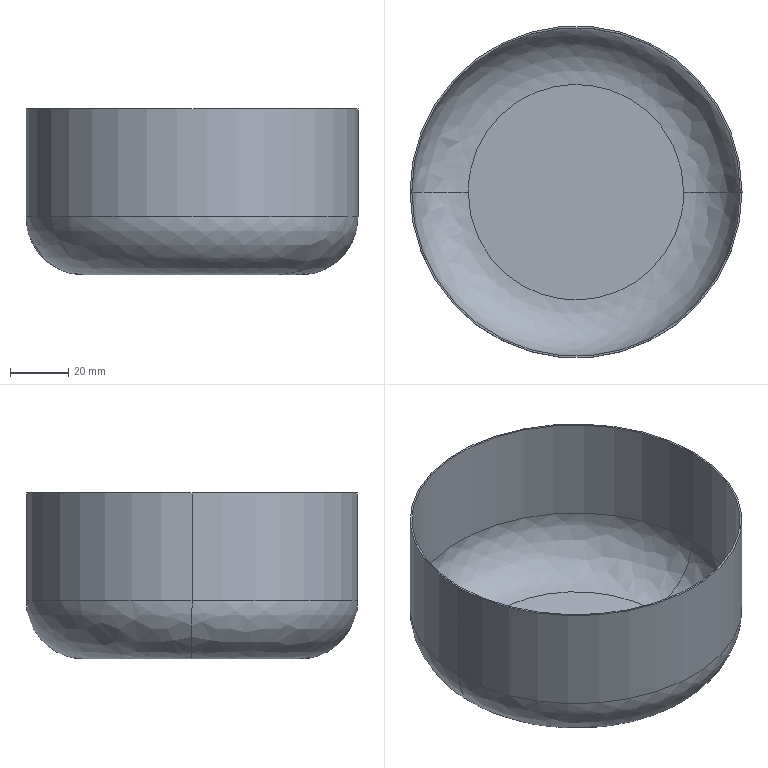Part | SolidWorks | features BaseBody 1 | 1 solid | 11 faces | box 114 x 114 x 57 mm | volume 16251 mm3 | spline 4 | cylinder 4 | plane 3 | commonest cylinder face diameters 112.8 x2 114 x2
STEP:
#1=CARTESIAN_POINT('',(-57.,0.,17.));
#2=VERTEX_POINT('',#1);
#3=CARTESIAN_POINT('',(57.,0.,17.));
#4=VERTEX_POINT('',#3);
#5=CARTESIAN_POINT('',(0.,0.,17.));
#6=DIRECTION('',(0.,0.,1.));
#7=DIRECTION('',(-1.,0.,0.));
#8=AXIS2_PLACEMENT_3D('',#5,#6,#7);
#9=CIRCLE('',#8,57.);
#10=EDGE_CURVE('',#2,#4,#9,.T.);
#11=ORIENTED_EDGE('',*,*,#10,.F.);
#12=CARTESIAN_POINT('',(-37.,0.,-3.));
#13=VERTEX_POINT('',#12);
#14=CARTESIAN_POINT('',(-37.,0.,17.));
#15=DIRECTION('',(0.,-1.,0.));
#16=DIRECTION('',(-1.,0.,0.));
#17=AXIS2_PLACEMENT_3D('',#14,#15,#16);
#18=CIRCLE('',#17,20.);
#19=EDGE_CURVE('',#2,#13,#18,.T.);
#20=ORIENTED_EDGE('',*,*,#19,.T.);
#21=CARTESIAN_POINT('',(37.,0.,-3.));
#22=VERTEX_POINT('',#21);
#23=CARTESIAN_POINT('',(-37.,0.,-3.));
#24=CARTESIAN_POINT('',(-37.,-74.,-3.));
#25=CARTESIAN_POINT('',(37.,-74.,-3.));
#26=CARTESIAN_POINT('',(37.,0.,-3.));
#27=(BOUNDED_CURVE()B_SPLINE_CURVE(3,(#23,#24,#25,#26),.UNSPECIFIED.,.F.,.F.)B_SPLINE_CURVE_WITH_KNOTS((4,4),(0.5,1.),.UNSPECIFIED.)CURVE()GEOMETRIC_REPRESENTATION_ITEM()RATIONAL_B_SPLINE_CURVE((1.,0.3333,0.3333,1.))REPRESENTATION_ITEM(''));
#28=EDGE_CURVE('',#13,#22,#27,.T.);
#29=ORIENTED_EDGE('',*,*,#28,.T.);
#30=CARTESIAN_POINT('',(37.,0.,17.));
#31=DIRECTION('',(0.,1.,0.));
#32=DIRECTION('',(1.,0.,0.));
#33=AXIS2_PLACEMENT_3D('',#30,#31,#32);
#34=CIRCLE('',#33,20.);
#35=EDGE_CURVE('',#4,#22,#34,.T.);
#36=ORIENTED_EDGE('',*,*,#35,.F.);
#37=EDGE_LOOP('',(#11,#20,#29,#36));
#38=FACE_OUTER_BOUND('',#37,.T.);
#39=CARTESIAN_POINT('',(-57.,0.,17.));
#40=CARTESIAN_POINT('',(-57.,-114.,17.));
#41=CARTESIAN_POINT('',(57.,-114.,17.));
#42=CARTESIAN_POINT('',(57.,0.,17.));
#43=CARTESIAN_POINT('',(-57.,0.,5.284));
#44=CARTESIAN_POINT('',(-57.,-114.,5.284));
#45=CARTESIAN_POINT('',(57.,-114.,5.284));
#46=CARTESIAN_POINT('',(57.,0.,5.284));
#47=CARTESIAN_POINT('',(-48.716,0.,-3.));
#48=CARTESIAN_POINT('',(-48.716,-97.431,-3.));
#49=CARTESIAN_POINT('',(48.716,-97.431,-3.));
#50=CARTESIAN_POINT('',(48.716,0.,-3.));
#51=CARTESIAN_POINT('',(-37.,0.,-3.));
#52=CARTESIAN_POINT('',(-37.,-74.,-3.));
#53=CARTESIAN_POINT('',(37.,-74.,-3.));
#54=CARTESIAN_POINT('',(37.,0.,-3.));
#55=(BOUNDED_SURFACE()B_SPLINE_SURFACE(3,3,((#39,#40,#41,#42),(#43,#44,#45,#46),(#47,#48,#49,#50),(#51,#52,#53,#54)),.UNSPECIFIED.,.F.,.F.,.F.)B_SPLINE_SURFACE_WITH_KNOTS((4,4),(4,4),(0.,1.),(0.,1.),.UNSPECIFIED.)GEOMETRIC_REPRESENTATION_ITEM()RATIONAL_B_SPLINE_SURFACE(((1.,0.3333,0.3333,1.),(0.8047,0.2682,0.2682,0.8047),(0.8047,0.2682,0.2682,0.8047),(1.,0.3333,0.3333,1.)))REPRESENTATION_ITEM('')SURFACE());
#56=ADVANCED_FACE('',(#38),#55,.T.);
#57=CARTESIAN_POINT('',(56.4,0.,17.));
#58=VERTEX_POINT('',#57);
#59=CARTESIAN_POINT('',(-56.4,0.,17.));
#60=VERTEX_POINT('',#59);
#61=CARTESIAN_POINT('',(0.,0.,17.));
#62=DIRECTION('',(0.,0.,1.));
#63=DIRECTION('',(-1.,0.,0.));
#64=AXIS2_PLACEMENT_3D('',#61,#62,#63);
#65=CIRCLE('',#64,56.4);
#66=EDGE_CURVE('',#58,#60,#65,.T.);
#67=ORIENTED_EDGE('',*,*,#66,.T.);
#68=CARTESIAN_POINT('',(-37.,0.,-2.4));
#69=VERTEX_POINT('',#68);
#70=CARTESIAN_POINT('',(-37.,0.,17.));
#71=DIRECTION('',(0.,-1.,0.));
#72=DIRECTION('',(-1.,0.,0.));
#73=AXIS2_PLACEMENT_3D('',#70,#71,#72);
#74=CIRCLE('',#73,19.4);
#75=EDGE_CURVE('',#60,#69,#74,.T.);
#76=ORIENTED_EDGE('',*,*,#75,.T.);
#77=CARTESIAN_POINT('',(37.,0.,-2.4));
#78=VERTEX_POINT('',#77);
#79=CARTESIAN_POINT('',(37.,0.,-2.4));
#80=CARTESIAN_POINT('',(37.,1.131,-2.4));
#81=CARTESIAN_POINT('',(36.923,2.822,-2.4));
#82=CARTESIAN_POINT('',(36.698,4.781,-2.4));
#83=CARTESIAN_POINT('',(36.551,5.758,-2.4));
#84=CARTESIAN_POINT('',(36.47,6.246,-2.4));
#85=CARTESIAN_POINT('',(36.427,6.489,-2.4));
#86=CARTESIAN_POINT('',(36.408,6.594,-2.4));
#87=CARTESIAN_POINT('',(36.395,6.663,-2.4));
#88=CARTESIAN_POINT('',(36.389,6.696,-2.4));
#89=CARTESIAN_POINT('',(36.164,7.912,-2.4));
#90=CARTESIAN_POINT('',(35.753,9.658,-2.4));
#91=CARTESIAN_POINT('',(35.126,11.653,-2.4));
#92=CARTESIAN_POINT('',(34.776,12.64,-2.4));
#93=CARTESIAN_POINT('',(34.592,13.13,-2.4));
#94=CARTESIAN_POINT('',(34.498,13.375,-2.4));
#95=CARTESIAN_POINT('',(34.457,13.48,-2.4));
#96=CARTESIAN_POINT('',(34.43,13.55,-2.4));
#97=CARTESIAN_POINT('',(34.417,13.583,-2.4));
#98=CARTESIAN_POINT('',(33.942,14.782,-2.4));
#99=CARTESIAN_POINT('',(33.168,16.482,-2.4));
#100=CARTESIAN_POINT('',(32.117,18.39,-2.4));
#101=CARTESIAN_POINT('',(31.555,19.325,-2.4));
#102=CARTESIAN_POINT('',(31.265,19.787,-2.4));
#103=CARTESIAN_POINT('',(31.139,19.985,-2.4));
#104=CARTESIAN_POINT('',(31.054,20.116,-2.4));
#105=CARTESIAN_POINT('',(31.013,20.18,-2.4));
#106=CARTESIAN_POINT('',(29.571,22.384,-2.4));
#107=CARTESIAN_POINT('',(27.969,24.357,-2.4));
#108=CARTESIAN_POINT('',(25.26,27.066,-2.4));
#109=CARTESIAN_POINT('',(23.843,28.344,-2.4));
#110=CARTESIAN_POINT('',(22.081,29.701,-2.4));
#111=CARTESIAN_POINT('',(21.173,30.346,-2.4));
#112=CARTESIAN_POINT('',(20.712,30.66,-2.4));
#113=CARTESIAN_POINT('',(20.513,30.793,-2.4));
#114=CARTESIAN_POINT('',(20.38,30.881,-2.4));
#115=CARTESIAN_POINT('',(20.312,30.926,-2.4));
#116=CARTESIAN_POINT('',(19.2,31.653,-2.4));
#117=CARTESIAN_POINT('',(17.587,32.595,-2.4));
#118=CARTESIAN_POINT('',(15.629,33.548,-2.4));
#119=CARTESIAN_POINT('',(14.631,33.987,-2.4));
#120=CARTESIAN_POINT('',(14.127,34.198,-2.4));
#121=CARTESIAN_POINT('',(13.873,34.301,-2.4));
#122=CARTESIAN_POINT('',(13.765,34.344,-2.4));
#123=CARTESIAN_POINT('',(13.692,34.373,-2.4));
#124=CARTESIAN_POINT('',(13.654,34.388,-2.4));
#125=CARTESIAN_POINT('',(12.504,34.844,-2.4));
#126=CARTESIAN_POINT('',(10.806,35.423,-2.4));
#127=CARTESIAN_POINT('',(8.784,35.951,-2.4));
#128=CARTESIAN_POINT('',(7.762,36.179,-2.4));
#129=CARTESIAN_POINT('',(7.248,36.284,-2.4));
#130=CARTESIAN_POINT('',(6.991,36.334,-2.4));
#131=CARTESIAN_POINT('',(6.88,36.355,-2.4));
#132=CARTESIAN_POINT('',(6.806,36.369,-2.4));
#133=CARTESIAN_POINT('',(6.767,36.376,-2.4));
#134=CARTESIAN_POINT('',(4.508,36.794,-2.4));
#135=CARTESIAN_POINT('',(2.263,37.,-2.4));
#136=CARTESIAN_POINT('',(-1.131,37.,-2.4));
#137=CARTESIAN_POINT('',(-2.821,36.923,-2.4));
#138=CARTESIAN_POINT('',(-4.781,36.698,-2.4));
#139=CARTESIAN_POINT('',(-5.758,36.551,-2.4));
#140=CARTESIAN_POINT('',(-6.246,36.47,-2.4));
#141=CARTESIAN_POINT('',(-6.489,36.427,-2.4));
#142=CARTESIAN_POINT('',(-6.594,36.408,-2.4));
#143=CARTESIAN_POINT('',(-6.663,36.395,-2.4));
#144=CARTESIAN_POINT('',(-6.696,36.389,-2.4));
#145=CARTESIAN_POINT('',(-7.912,36.164,-2.4));
#146=CARTESIAN_POINT('',(-9.658,35.753,-2.4));
#147=CARTESIAN_POINT('',(-11.653,35.126,-2.4));
#148=CARTESIAN_POINT('',(-12.64,34.776,-2.4));
#149=CARTESIAN_POINT('',(-13.13,34.592,-2.4));
#150=CARTESIAN_POINT('',(-13.375,34.498,-2.4));
#151=CARTESIAN_POINT('',(-13.48,34.457,-2.4));
#152=CARTESIAN_POINT('',(-13.55,34.43,-2.4));
#153=CARTESIAN_POINT('',(-13.583,34.417,-2.4));
#154=CARTESIAN_POINT('',(-14.782,33.942,-2.4));
#155=CARTESIAN_POINT('',(-16.482,33.168,-2.4));
#156=CARTESIAN_POINT('',(-18.39,32.117,-2.4));
#157=CARTESIAN_POINT('',(-19.325,31.555,-2.4));
#158=CARTESIAN_POINT('',(-19.787,31.265,-2.4));
#159=CARTESIAN_POINT('',(-19.985,31.139,-2.4));
#160=CARTESIAN_POINT('',(-20.116,31.054,-2.4));
#161=CARTESIAN_POINT('',(-20.18,31.013,-2.4));
#162=CARTESIAN_POINT('',(-22.384,29.571,-2.4));
#163=CARTESIAN_POINT('',(-24.357,27.969,-2.4));
#164=CARTESIAN_POINT('',(-27.066,25.26,-2.4));
#165=CARTESIAN_POINT('',(-28.344,23.843,-2.4));
#166=CARTESIAN_POINT('',(-29.701,22.081,-2.4));
#167=CARTESIAN_POINT('',(-30.346,21.173,-2.4));
#168=CARTESIAN_POINT('',(-30.66,20.712,-2.4));
#169=CARTESIAN_POINT('',(-30.793,20.513,-2.4));
#170=CARTESIAN_POINT('',(-30.881,20.38,-2.4));
#171=CARTESIAN_POINT('',(-30.926,20.312,-2.4));
#172=CARTESIAN_POINT('',(-31.653,19.2,-2.4));
#173=CARTESIAN_POINT('',(-32.595,17.587,-2.4));
#174=CARTESIAN_POINT('',(-33.548,15.629,-2.4));
#175=CARTESIAN_POINT('',(-33.987,14.631,-2.4));
#176=CARTESIAN_POINT('',(-34.198,14.127,-2.4));
#177=CARTESIAN_POINT('',(-34.301,13.873,-2.4));
#178=CARTESIAN_POINT('',(-34.344,13.765,-2.4));
#179=CARTESIAN_POINT('',(-34.373,13.692,-2.4));
#180=CARTESIAN_POINT('',(-34.388,13.654,-2.4));
#181=CARTESIAN_POINT('',(-34.844,12.504,-2.4));
#182=CARTESIAN_POINT('',(-35.423,10.806,-2.4));
#183=CARTESIAN_POINT('',(-35.951,8.784,-2.4));
#184=CARTESIAN_POINT('',(-36.179,7.762,-2.4));
#185=CARTESIAN_POINT('',(-36.284,7.248,-2.4));
#186=CARTESIAN_POINT('',(-36.334,6.991,-2.4));
#187=CARTESIAN_POINT('',(-36.355,6.88,-2.4));
#188=CARTESIAN_POINT('',(-36.369,6.806,-2.4));
#189=CARTESIAN_POINT('',(-36.376,6.767,-2.4));
#190=CARTESIAN_POINT('',(-36.794,4.508,-2.4));
#191=CARTESIAN_POINT('',(-37.,2.263,-2.4));
#192=CARTESIAN_POINT('',(-37.,0.,-2.4));
#193=B_SPLINE_CURVE_WITH_KNOTS('',3,(#79,#80,#81,#82,#83,#84,#85,#86,#87,#88,#89,#90,#91,#92,#93,#94,#95,#96,#97,#98,#99,#100,#101,#102,#103,#104,#105,#106,#107,#108,#109,#110,#111,#112,#113,#114,#115,#116,#117,#118,#119,#120,#121,#122,#123,#124,#125,#126,#127,#128,#129,#130,#131,#132,#133,#134,#135,#136,#137,#138,#139,#140,#141,#142,#143,#144,#145,#146,#147,#148,#149,#150,#151,#152,#153,#154,#155,#156,#157,#158,#159,#160,#161,#162,#163,#164,#165,#166,#167,#168,#169,#170,#171,#172,#173,#174,#175,#176,#177,#178,#179,#180,#181,#182,#183,#184,#185,#186,#187,#188,#189,#190,#191,#192),.UNSPECIFIED.,.F.,.F.,(4,1,1,1,1,1,2,2,1,1,1,1,1,2,2,1,1,1,1,2,2,2,1,1,1,1,2,2,1,1,1,1,1,2,2,1,1,1,1,1,2,2,2,1,1,1,1,1,2,2,1,1,1,1,1,2,2,1,1,1,1,2,2,2,1,1,1,1,2,2,1,1,1,1,1,2,2,1,1,1,1,1,2,2,4),(0.,0.01563,0.02344,0.02734,0.0293,0.03027,0.03076,0.03125,0.04688,0.05469,0.05859,0.06055,0.06152,0.06201,0.0625,0.07813,0.08594,0.08984,0.0918,0.09277,0.09375,0.125,0.1406,0.1484,0.1523,0.1543,0.1553,0.1563,0.1719,0.1797,0.1836,0.1855,0.1865,0.187,0.1875,0.2031,0.2109,0.2148,0.2168,0.2178,0.2183,0.2188,0.25,0.2656,0.2734,0.2773,0.2793,0.2803,0.2808,0.2813,0.2969,0.3047,0.3086,0.3105,0.3115,0.312,0.3125,0.3281,0.3359,0.3398,0.3418,0.3428,0.3438,0.375,0.3906,0.3984,0.4023,0.4043,0.4053,0.4063,0.4219,0.4297,0.4336,0.4355,0.4365,0.437,0.4375,0.4531,0.4609,0.4648,0.4668,0.4678,0.4683,0.4688,0.5),.UNSPECIFIED.);
#194=EDGE_CURVE('',#78,#69,#193,.T.);
#195=ORIENTED_EDGE('',*,*,#194,.F.);
#196=CARTESIAN_POINT('',(37.,0.,17.));
#197=DIRECTION('',(0.,1.,0.));
#198=DIRECTION('',(1.,0.,0.));
#199=AXIS2_PLACEMENT_3D('',#196,#197,#198);
#200=CIRCLE('',#199,19.4);
#201=EDGE_CURVE('',#58,#78,#200,.T.);
#202=ORIENTED_EDGE('',*,*,#201,.F.);
#203=EDGE_LOOP('',(#67,#76,#195,#202));
#204=FACE_OUTER_BOUND('',#203,.T.);
#205=CARTESIAN_POINT('',(56.4,0.,17.));
#206=CARTESIAN_POINT('',(56.4,112.8,17.));
#207=CARTESIAN_POINT('',(-56.4,112.8,17.));
#208=CARTESIAN_POINT('',(-56.4,0.,17.));
#209=CARTESIAN_POINT('',(56.4,0.,5.636));
#210=CARTESIAN_POINT('',(56.4,112.8,5.636));
#211=CARTESIAN_POINT('',(-56.4,112.8,5.636));
#212=CARTESIAN_POINT('',(-56.4,0.,5.636));
#213=CARTESIAN_POINT('',(48.364,0.,-2.4));
#214=CARTESIAN_POINT('',(48.364,96.729,-2.4));
#215=CARTESIAN_POINT('',(-48.364,96.729,-2.4));
#216=CARTESIAN_POINT('',(-48.364,0.,-2.4));
#217=CARTESIAN_POINT('',(37.,0.,-2.4));
#218=CARTESIAN_POINT('',(37.,74.,-2.4));
#219=CARTESIAN_POINT('',(-37.,74.,-2.4));
#220=CARTESIAN_POINT('',(-37.,0.,-2.4));
#221=(BOUNDED_SURFACE()B_SPLINE_SURFACE(3,3,((#205,#206,#207,#208),(#209,#210,#211,#212),(#213,#214,#215,#216),(#217,#218,#219,#220)),.UNSPECIFIED.,.F.,.F.,.F.)B_SPLINE_SURFACE_WITH_KNOTS((4,4),(4,4),(0.,1.),(0.,1.),.UNSPECIFIED.)GEOMETRIC_REPRESENTATION_ITEM()RATIONAL_B_SPLINE_SURFACE(((1.,0.3333,0.3333,1.),(0.8047,0.2682,0.2682,0.8047),(0.8047,0.2682,0.2682,0.8047),(1.,0.3333,0.3333,1.)))REPRESENTATION_ITEM('')SURFACE());
#222=ADVANCED_FACE('',(#204),#221,.F.);
#223=CARTESIAN_POINT('',(-57.,0.,54.));
#224=VERTEX_POINT('',#223);
#225=CARTESIAN_POINT('',(57.,0.,54.));
#226=VERTEX_POINT('',#225);
#227=CARTESIAN_POINT('',(0.,0.,54.));
#228=DIRECTION('',(0.,0.,-1.));
#229=DIRECTION('',(-1.,0.,0.));
#230=AXIS2_PLACEMENT_3D('',#227,#228,#229);
#231=CIRCLE('',#230,57.);
#232=EDGE_CURVE('',#224,#226,#231,.T.);
#233=ORIENTED_EDGE('',*,*,#232,.T.);
#234=CARTESIAN_POINT('',(57.,0.,54.));
#235=DIRECTION('',(0.,0.,-1.));
#236=VECTOR('',#235,1000.);
#237=LINE('',#234,#236);
#238=EDGE_CURVE('',#226,#4,#237,.T.);
#239=ORIENTED_EDGE('',*,*,#238,.T.);
#240=CARTESIAN_POINT('',(0.,0.,17.));
#241=DIRECTION('',(0.,0.,1.));
#242=DIRECTION('',(-1.,0.,0.));
#243=AXIS2_PLACEMENT_3D('',#240,#241,#242);
#244=CIRCLE('',#243,57.);
#245=EDGE_CURVE('',#4,#2,#244,.T.);
#246=ORIENTED_EDGE('',*,*,#245,.T.);
#247=CARTESIAN_POINT('',(-57.,0.,54.));
#248=DIRECTION('',(0.,0.,-1.));
#249=VECTOR('',#248,1000.);
#250=LINE('',#247,#249);
#251=EDGE_CURVE('',#224,#2,#250,.T.);
#252=ORIENTED_EDGE('',*,*,#251,.F.);
#253=EDGE_LOOP('',(#233,#239,#246,#252));
#254=FACE_OUTER_BOUND('',#253,.T.);
#255=CARTESIAN_POINT('',(0.,0.,54.));
#256=DIRECTION('',(0.,0.,-1.));
#257=DIRECTION('',(-1.,0.,0.));
#258=AXIS2_PLACEMENT_3D('',#255,#256,#257);
#259=CYLINDRICAL_SURFACE('',#258,57.);
#260=ADVANCED_FACE('',(#254),#259,.T.);
#261=CARTESIAN_POINT('',(56.4,0.,54.));
#262=VERTEX_POINT('',#261);
#263=CARTESIAN_POINT('',(-56.4,0.,54.));
#264=VERTEX_POINT('',#263);
#265=CARTESIAN_POINT('',(0.,0.,54.));
#266=DIRECTION('',(0.,0.,-1.));
#267=DIRECTION('',(-1.,0.,0.));
#268=AXIS2_PLACEMENT_3D('',#265,#266,#267);
#269=CIRCLE('',#268,56.4);
#270=EDGE_CURVE('',#262,#264,#269,.T.);
#271=ORIENTED_EDGE('',*,*,#270,.F.);
#272=CARTESIAN_POINT('',(56.4,0.,54.));
#273=DIRECTION('',(0.,0.,-1.));
#274=VECTOR('',#273,1000.);
#275=LINE('',#272,#274);
#276=EDGE_CURVE('',#262,#58,#275,.T.);
#277=ORIENTED_EDGE('',*,*,#276,.T.);
#278=CARTESIAN_POINT('',(0.,0.,17.));
#279=DIRECTION('',(0.,0.,1.));
#280=DIRECTION('',(-1.,0.,0.));
#281=AXIS2_PLACEMENT_3D('',#278,#279,#280);
#282=CIRCLE('',#281,56.4);
#283=EDGE_CURVE('',#60,#58,#282,.T.);
#284=ORIENTED_EDGE('',*,*,#283,.F.);
#285=CARTESIAN_POINT('',(-56.4,0.,54.));
#286=DIRECTION('',(0.,0.,-1.));
#287=VECTOR('',#286,1000.);
#288=LINE('',#285,#287);
#289=EDGE_CURVE('',#264,#60,#288,.T.);
#290=ORIENTED_EDGE('',*,*,#289,.F.);
#291=EDGE_LOOP('',(#271,#277,#284,#290));
#292=FACE_OUTER_BOUND('',#291,.T.);
#293=CARTESIAN_POINT('',(0.,0.,54.));
#294=DIRECTION('',(0.,0.,-1.));
#295=DIRECTION('',(-1.,0.,0.));
#296=AXIS2_PLACEMENT_3D('',#293,#294,#295);
#297=CYLINDRICAL_SURFACE('',#296,56.4);
#298=ADVANCED_FACE('',(#292),#297,.F.);
#299=ORIENTED_EDGE('',*,*,#238,.F.);
#300=CARTESIAN_POINT('',(0.,0.,54.));
#301=DIRECTION('',(0.,0.,-1.));
#302=DIRECTION('',(-1.,0.,0.));
#303=AXIS2_PLACEMENT_3D('',#300,#301,#302);
#304=CIRCLE('',#303,57.);
#305=EDGE_CURVE('',#226,#224,#304,.T.);
#306=ORIENTED_EDGE('',*,*,#305,.T.);
#307=ORIENTED_EDGE('',*,*,#251,.T.);
#308=ORIENTED_EDGE('',*,*,#10,.T.);
#309=EDGE_LOOP('',(#299,#306,#307,#308));
#310=FACE_OUTER_BOUND('',#309,.T.);
#311=CARTESIAN_POINT('',(0.,0.,54.));
#312=DIRECTION('',(0.,0.,-1.));
#313=DIRECTION('',(-1.,0.,0.));
#314=AXIS2_PLACEMENT_3D('',#311,#312,#313);
#315=CYLINDRICAL_SURFACE('',#314,57.);
#316=ADVANCED_FACE('',(#310),#315,.T.);
#317=ORIENTED_EDGE('',*,*,#232,.F.);
#318=ORIENTED_EDGE('',*,*,#305,.F.);
#319=EDGE_LOOP('',(#317,#318));
#320=FACE_OUTER_BOUND('',#319,.T.);
#321=CARTESIAN_POINT('',(0.,0.,54.));
#322=DIRECTION('',(0.,0.,-1.));
#323=DIRECTION('',(-1.,0.,0.));
#324=AXIS2_PLACEMENT_3D('',#321,#322,#323);
#325=CIRCLE('',#324,56.4);
#326=EDGE_CURVE('',#264,#262,#325,.T.);
#327=ORIENTED_EDGE('',*,*,#326,.T.);
#328=ORIENTED_EDGE('',*,*,#270,.T.);
#329=EDGE_LOOP('',(#327,#328));
#330=FACE_BOUND('',#329,.T.);
#331=CARTESIAN_POINT('',(0.,0.,54.));
#332=DIRECTION('',(0.,0.,1.));
#333=DIRECTION('',(1.,0.,0.));
#334=AXIS2_PLACEMENT_3D('',#331,#332,#333);
#335=PLANE('',#334);
#336=ADVANCED_FACE('',(#320,#330),#335,.T.);
#337=ORIENTED_EDGE('',*,*,#19,.F.);
#338=ORIENTED_EDGE('',*,*,#245,.F.);
#339=ORIENTED_EDGE('',*,*,#35,.T.);
#340=CARTESIAN_POINT('',(37.,0.,-3.));
#341=CARTESIAN_POINT('',(37.,74.,-3.));
#342=CARTESIAN_POINT('',(-37.,74.,-3.));
#343=CARTESIAN_POINT('',(-37.,0.,-3.));
#344=(BOUNDED_CURVE()B_SPLINE_CURVE(3,(#340,#341,#342,#343),.UNSPECIFIED.,.F.,.F.)B_SPLINE_CURVE_WITH_KNOTS((4,4),(0.,0.5),.UNSPECIFIED.)CURVE()GEOMETRIC_REPRESENTATION_ITEM()RATIONAL_B_SPLINE_CURVE((1.,0.3333,0.3333,1.))REPRESENTATION_ITEM(''));
#345=EDGE_CURVE('',#22,#13,#344,.T.);
#346=ORIENTED_EDGE('',*,*,#345,.T.);
#347=EDGE_LOOP('',(#337,#338,#339,#346));
#348=FACE_OUTER_BOUND('',#347,.T.);
#349=CARTESIAN_POINT('',(57.,0.,17.));
#350=CARTESIAN_POINT('',(57.,114.,17.));
#351=CARTESIAN_POINT('',(-57.,114.,17.));
#352=CARTESIAN_POINT('',(-57.,0.,17.));
#353=CARTESIAN_POINT('',(57.,0.,5.284));
#354=CARTESIAN_POINT('',(57.,114.,5.284));
#355=CARTESIAN_POINT('',(-57.,114.,5.284));
#356=CARTESIAN_POINT('',(-57.,0.,5.284));
#357=CARTESIAN_POINT('',(48.716,0.,-3.));
#358=CARTESIAN_POINT('',(48.716,97.431,-3.));
#359=CARTESIAN_POINT('',(-48.716,97.431,-3.));
#360=CARTESIAN_POINT('',(-48.716,0.,-3.));
#361=CARTESIAN_POINT('',(37.,0.,-3.));
#362=CARTESIAN_POINT('',(37.,74.,-3.));
#363=CARTESIAN_POINT('',(-37.,74.,-3.));
#364=CARTESIAN_POINT('',(-37.,0.,-3.));
#365=(BOUNDED_SURFACE()B_SPLINE_SURFACE(3,3,((#349,#350,#351,#352),(#353,#354,#355,#356),(#357,#358,#359,#360),(#361,#362,#363,#364)),.UNSPECIFIED.,.F.,.F.,.T.)B_SPLINE_SURFACE_WITH_KNOTS((4,4),(4,4),(0.,1.),(0.,1.),.UNSPECIFIED.)GEOMETRIC_REPRESENTATION_ITEM()RATIONAL_B_SPLINE_SURFACE(((1.,0.3333,0.3333,1.),(0.8047,0.2682,0.2682,0.8047),(0.8047,0.2682,0.2682,0.8047),(1.,0.3333,0.3333,1.)))REPRESENTATION_ITEM('')SURFACE());
#366=ADVANCED_FACE('',(#348),#365,.T.);
#367=ORIENTED_EDGE('',*,*,#276,.F.);
#368=ORIENTED_EDGE('',*,*,#326,.F.);
#369=ORIENTED_EDGE('',*,*,#289,.T.);
#370=ORIENTED_EDGE('',*,*,#66,.F.);
#371=EDGE_LOOP('',(#367,#368,#369,#370));
#372=FACE_OUTER_BOUND('',#371,.T.);
#373=CARTESIAN_POINT('',(0.,0.,54.));
#374=DIRECTION('',(0.,0.,-1.));
#375=DIRECTION('',(-1.,0.,0.));
#376=AXIS2_PLACEMENT_3D('',#373,#374,#375);
#377=CYLINDRICAL_SURFACE('',#376,56.4);
#378=ADVANCED_FACE('',(#372),#377,.F.);
#379=ORIENTED_EDGE('',*,*,#345,.F.);
#380=ORIENTED_EDGE('',*,*,#28,.F.);
#381=EDGE_LOOP('',(#379,#380));
#382=FACE_OUTER_BOUND('',#381,.T.);
#383=CARTESIAN_POINT('',(0.,0.,-3.));
#384=DIRECTION('',(0.,0.,1.));
#385=DIRECTION('',(1.,0.,0.));
#386=AXIS2_PLACEMENT_3D('',#383,#384,#385);
#387=PLANE('',#386);
#388=ADVANCED_FACE('',(#382),#387,.F.);
#389=ORIENTED_EDGE('',*,*,#75,.F.);
#390=ORIENTED_EDGE('',*,*,#283,.T.);
#391=ORIENTED_EDGE('',*,*,#201,.T.);
#392=CARTESIAN_POINT('',(-37.,0.,-2.4));
#393=CARTESIAN_POINT('',(-37.,-1.131,-2.4));
#394=CARTESIAN_POINT('',(-36.923,-2.821,-2.4));
#395=CARTESIAN_POINT('',(-36.698,-4.781,-2.4));
#396=CARTESIAN_POINT('',(-36.551,-5.758,-2.4));
#397=CARTESIAN_POINT('',(-36.47,-6.246,-2.4));
#398=CARTESIAN_POINT('',(-36.427,-6.489,-2.4));
#399=CARTESIAN_POINT('',(-36.408,-6.594,-2.4));
#400=CARTESIAN_POINT('',(-36.395,-6.663,-2.4));
#401=CARTESIAN_POINT('',(-36.389,-6.696,-2.4));
#402=CARTESIAN_POINT('',(-36.164,-7.912,-2.4));
#403=CARTESIAN_POINT('',(-35.753,-9.658,-2.4));
#404=CARTESIAN_POINT('',(-35.126,-11.653,-2.4));
#405=CARTESIAN_POINT('',(-34.776,-12.64,-2.4));
#406=CARTESIAN_POINT('',(-34.592,-13.13,-2.4));
#407=CARTESIAN_POINT('',(-34.498,-13.375,-2.4));
#408=CARTESIAN_POINT('',(-34.457,-13.48,-2.4));
#409=CARTESIAN_POINT('',(-34.43,-13.55,-2.4));
#410=CARTESIAN_POINT('',(-34.417,-13.583,-2.4));
#411=CARTESIAN_POINT('',(-33.942,-14.782,-2.4));
#412=CARTESIAN_POINT('',(-33.168,-16.482,-2.4));
#413=CARTESIAN_POINT('',(-32.117,-18.39,-2.4));
#414=CARTESIAN_POINT('',(-31.555,-19.325,-2.4));
#415=CARTESIAN_POINT('',(-31.265,-19.787,-2.4));
#416=CARTESIAN_POINT('',(-31.139,-19.985,-2.4));
#417=CARTESIAN_POINT('',(-31.054,-20.116,-2.4));
#418=CARTESIAN_POINT('',(-31.013,-20.18,-2.4));
#419=CARTESIAN_POINT('',(-29.571,-22.384,-2.4));
#420=CARTESIAN_POINT('',(-27.969,-24.357,-2.4));
#421=CARTESIAN_POINT('',(-25.26,-27.066,-2.4));
#422=CARTESIAN_POINT('',(-23.843,-28.344,-2.4));
#423=CARTESIAN_POINT('',(-22.081,-29.701,-2.4));
#424=CARTESIAN_POINT('',(-21.173,-30.346,-2.4));
#425=CARTESIAN_POINT('',(-20.712,-30.66,-2.4));
#426=CARTESIAN_POINT('',(-20.513,-30.793,-2.4));
#427=CARTESIAN_POINT('',(-20.38,-30.881,-2.4));
#428=CARTESIAN_POINT('',(-20.312,-30.926,-2.4));
#429=CARTESIAN_POINT('',(-19.2,-31.653,-2.4));
#430=CARTESIAN_POINT('',(-17.587,-32.595,-2.4));
#431=CARTESIAN_POINT('',(-15.629,-33.548,-2.4));
#432=CARTESIAN_POINT('',(-14.631,-33.987,-2.4));
#433=CARTESIAN_POINT('',(-14.127,-34.198,-2.4));
#434=CARTESIAN_POINT('',(-13.873,-34.301,-2.4));
#435=CARTESIAN_POINT('',(-13.765,-34.344,-2.4));
#436=CARTESIAN_POINT('',(-13.692,-34.373,-2.4));
#437=CARTESIAN_POINT('',(-13.654,-34.388,-2.4));
#438=CARTESIAN_POINT('',(-12.504,-34.844,-2.4));
#439=CARTESIAN_POINT('',(-10.806,-35.423,-2.4));
#440=CARTESIAN_POINT('',(-8.784,-35.951,-2.4));
#441=CARTESIAN_POINT('',(-7.762,-36.179,-2.4));
#442=CARTESIAN_POINT('',(-7.248,-36.284,-2.4));
#443=CARTESIAN_POINT('',(-6.991,-36.334,-2.4));
#444=CARTESIAN_POINT('',(-6.88,-36.355,-2.4));
#445=CARTESIAN_POINT('',(-6.806,-36.369,-2.4));
#446=CARTESIAN_POINT('',(-6.767,-36.376,-2.4));
#447=CARTESIAN_POINT('',(-4.508,-36.794,-2.4));
#448=CARTESIAN_POINT('',(-2.263,-37.,-2.4));
#449=CARTESIAN_POINT('',(1.131,-37.,-2.4));
#450=CARTESIAN_POINT('',(2.821,-36.923,-2.4));
#451=CARTESIAN_POINT('',(4.781,-36.698,-2.4));
#452=CARTESIAN_POINT('',(5.758,-36.551,-2.4));
#453=CARTESIAN_POINT('',(6.246,-36.47,-2.4));
#454=CARTESIAN_POINT('',(6.489,-36.427,-2.4));
#455=CARTESIAN_POINT('',(6.594,-36.408,-2.4));
#456=CARTESIAN_POINT('',(6.663,-36.395,-2.4));
#457=CARTESIAN_POINT('',(6.696,-36.389,-2.4));
#458=CARTESIAN_POINT('',(7.912,-36.164,-2.4));
#459=CARTESIAN_POINT('',(9.658,-35.753,-2.4));
#460=CARTESIAN_POINT('',(11.653,-35.126,-2.4));
#461=CARTESIAN_POINT('',(12.64,-34.776,-2.4));
#462=CARTESIAN_POINT('',(13.13,-34.592,-2.4));
#463=CARTESIAN_POINT('',(13.375,-34.498,-2.4));
#464=CARTESIAN_POINT('',(13.48,-34.457,-2.4));
#465=CARTESIAN_POINT('',(13.55,-34.43,-2.4));
#466=CARTESIAN_POINT('',(13.583,-34.417,-2.4));
#467=CARTESIAN_POINT('',(14.782,-33.942,-2.4));
#468=CARTESIAN_POINT('',(16.482,-33.168,-2.4));
#469=CARTESIAN_POINT('',(18.39,-32.117,-2.4));
#470=CARTESIAN_POINT('',(19.325,-31.555,-2.4));
#471=CARTESIAN_POINT('',(19.787,-31.265,-2.4));
#472=CARTESIAN_POINT('',(19.985,-31.139,-2.4));
#473=CARTESIAN_POINT('',(20.116,-31.054,-2.4));
#474=CARTESIAN_POINT('',(20.18,-31.013,-2.4));
#475=CARTESIAN_POINT('',(22.384,-29.571,-2.4));
#476=CARTESIAN_POINT('',(24.357,-27.969,-2.4));
#477=CARTESIAN_POINT('',(27.066,-25.26,-2.4));
#478=CARTESIAN_POINT('',(28.344,-23.843,-2.4));
#479=CARTESIAN_POINT('',(29.701,-22.081,-2.4));
#480=CARTESIAN_POINT('',(30.346,-21.173,-2.4));
#481=CARTESIAN_POINT('',(30.66,-20.712,-2.4));
#482=CARTESIAN_POINT('',(30.793,-20.513,-2.4));
#483=CARTESIAN_POINT('',(30.881,-20.38,-2.4));
#484=CARTESIAN_POINT('',(30.926,-20.312,-2.4));
#485=CARTESIAN_POINT('',(31.653,-19.2,-2.4));
#486=CARTESIAN_POINT('',(32.595,-17.587,-2.4));
#487=CARTESIAN_POINT('',(33.548,-15.629,-2.4));
#488=CARTESIAN_POINT('',(33.987,-14.631,-2.4));
#489=CARTESIAN_POINT('',(34.198,-14.127,-2.4));
#490=CARTESIAN_POINT('',(34.301,-13.873,-2.4));
#491=CARTESIAN_POINT('',(34.344,-13.765,-2.4));
#492=CARTESIAN_POINT('',(34.373,-13.692,-2.4));
#493=CARTESIAN_POINT('',(34.388,-13.654,-2.4));
#494=CARTESIAN_POINT('',(34.844,-12.504,-2.4));
#495=CARTESIAN_POINT('',(35.423,-10.806,-2.4));
#496=CARTESIAN_POINT('',(35.951,-8.784,-2.4));
#497=CARTESIAN_POINT('',(36.179,-7.762,-2.4));
#498=CARTESIAN_POINT('',(36.284,-7.248,-2.4));
#499=CARTESIAN_POINT('',(36.334,-6.991,-2.4));
#500=CARTESIAN_POINT('',(36.355,-6.88,-2.4));
#501=CARTESIAN_POINT('',(36.369,-6.806,-2.4));
#502=CARTESIAN_POINT('',(36.376,-6.767,-2.4));
#503=CARTESIAN_POINT('',(36.794,-4.507,-2.4));
#504=CARTESIAN_POINT('',(37.,-2.263,-2.4));
#505=CARTESIAN_POINT('',(37.,0.,-2.4));
#506=B_SPLINE_CURVE_WITH_KNOTS('',3,(#392,#393,#394,#395,#396,#397,#398,#399,#400,#401,#402,#403,#404,#405,#406,#407,#408,#409,#410,#411,#412,#413,#414,#415,#416,#417,#418,#419,#420,#421,#422,#423,#424,#425,#426,#427,#428,#429,#430,#431,#432,#433,#434,#435,#436,#437,#438,#439,#440,#441,#442,#443,#444,#445,#446,#447,#448,#449,#450,#451,#452,#453,#454,#455,#456,#457,#458,#459,#460,#461,#462,#463,#464,#465,#466,#467,#468,#469,#470,#471,#472,#473,#474,#475,#476,#477,#478,#479,#480,#481,#482,#483,#484,#485,#486,#487,#488,#489,#490,#491,#492,#493,#494,#495,#496,#497,#498,#499,#500,#501,#502,#503,#504,#505),.UNSPECIFIED.,.F.,.F.,(4,1,1,1,1,1,2,2,1,1,1,1,1,2,2,1,1,1,1,2,2,2,1,1,1,1,2,2,1,1,1,1,1,2,2,1,1,1,1,1,2,2,2,1,1,1,1,1,2,2,1,1,1,1,1,2,2,1,1,1,1,2,2,2,1,1,1,1,2,2,1,1,1,1,1,2,2,1,1,1,1,1,2,2,4),(0.5,0.5156,0.5234,0.5273,0.5293,0.5303,0.5308,0.5312,0.5469,0.5547,0.5586,0.5605,0.5615,0.562,0.5625,0.5781,0.5859,0.5898,0.5918,0.5928,0.5937,0.625,0.6406,0.6484,0.6523,0.6543,0.6553,0.6562,0.6719,0.6797,0.6836,0.6855,0.6865,0.687,0.6875,0.7031,0.7109,0.7148,0.7168,0.7178,0.7183,0.7187,0.75,0.7656,0.7734,0.7773,0.7793,0.7803,0.7808,0.7812,0.7969,0.8047,0.8086,0.8105,0.8115,0.812,0.8125,0.8281,0.8359,0.8398,0.8418,0.8428,0.8437,0.875,0.8906,0.8984,0.9023,0.9043,0.9053,0.9062,0.9219,0.9297,0.9336,0.9355,0.9365,0.937,0.9375,0.9531,0.9609,0.9648,0.9668,0.9678,0.9683,0.9687,1.),.UNSPECIFIED.);
#507=EDGE_CURVE('',#69,#78,#506,.T.);
#508=ORIENTED_EDGE('',*,*,#507,.F.);
#509=EDGE_LOOP('',(#389,#390,#391,#508));
#510=FACE_OUTER_BOUND('',#509,.T.);
#511=CARTESIAN_POINT('',(-56.4,0.,17.));
#512=CARTESIAN_POINT('',(-56.4,-112.8,17.));
#513=CARTESIAN_POINT('',(56.4,-112.8,17.));
#514=CARTESIAN_POINT('',(56.4,0.,17.));
#515=CARTESIAN_POINT('',(-56.4,0.,5.636));
#516=CARTESIAN_POINT('',(-56.4,-112.8,5.636));
#517=CARTESIAN_POINT('',(56.4,-112.8,5.636));
#518=CARTESIAN_POINT('',(56.4,0.,5.636));
#519=CARTESIAN_POINT('',(-48.364,0.,-2.4));
#520=CARTESIAN_POINT('',(-48.364,-96.729,-2.4));
#521=CARTESIAN_POINT('',(48.364,-96.729,-2.4));
#522=CARTESIAN_POINT('',(48.364,0.,-2.4));
#523=CARTESIAN_POINT('',(-37.,0.,-2.4));
#524=CARTESIAN_POINT('',(-37.,-74.,-2.4));
#525=CARTESIAN_POINT('',(37.,-74.,-2.4));
#526=CARTESIAN_POINT('',(37.,0.,-2.4));
#527=(BOUNDED_SURFACE()B_SPLINE_SURFACE(3,3,((#511,#512,#513,#514),(#515,#516,#517,#518),(#519,#520,#521,#522),(#523,#524,#525,#526)),.UNSPECIFIED.,.F.,.F.,.T.)B_SPLINE_SURFACE_WITH_KNOTS((4,4),(4,4),(0.,1.),(0.,1.),.UNSPECIFIED.)GEOMETRIC_REPRESENTATION_ITEM()RATIONAL_B_SPLINE_SURFACE(((1.,0.3333,0.3333,1.),(0.8047,0.2682,0.2682,0.8047),(0.8047,0.2682,0.2682,0.8047),(1.,0.3333,0.3333,1.)))REPRESENTATION_ITEM('')SURFACE());
#528=ADVANCED_FACE('',(#510),#527,.F.);
#529=ORIENTED_EDGE('',*,*,#194,.T.);
#530=ORIENTED_EDGE('',*,*,#507,.T.);
#531=EDGE_LOOP('',(#529,#530));
#532=FACE_OUTER_BOUND('',#531,.T.);
#533=CARTESIAN_POINT('',(0.,0.,-2.4));
#534=DIRECTION('',(0.,0.,1.));
#535=DIRECTION('',(1.,0.,0.));
#536=AXIS2_PLACEMENT_3D('',#533,#534,#535);
#537=PLANE('',#536);
#538=ADVANCED_FACE('',(#532),#537,.T.);
#539=CLOSED_SHELL('',(#56,#222,#260,#298,#316,#336,#366,#378,#388,#528,#538));
#540=MANIFOLD_SOLID_BREP('',#539);
#541=CARTESIAN_POINT('',(0.,0.,0.));
#542=DIRECTION('',(0.,0.,1.));
#543=DIRECTION('',(1.,0.,0.));
#544=AXIS2_PLACEMENT_3D('',#541,#542,#543);
#545=(LENGTH_UNIT()NAMED_UNIT(*)SI_UNIT(.MILLI.,.METRE.));
#546=UNCERTAINTY_MEASURE_WITH_UNIT(LENGTH_MEASURE(0.00001),#545,'','');
#547=(NAMED_UNIT(*)PLANE_ANGLE_UNIT()SI_UNIT($,.RADIAN.));
#548=(NAMED_UNIT(*)SI_UNIT($,.STERADIAN.)SOLID_ANGLE_UNIT());
#549=(GEOMETRIC_REPRESENTATION_CONTEXT(3)GLOBAL_UNCERTAINTY_ASSIGNED_CONTEXT((#546))GLOBAL_UNIT_ASSIGNED_CONTEXT((#545,#547,#548))REPRESENTATION_CONTEXT('',''));
#550=ADVANCED_BREP_SHAPE_REPRESENTATION('',(#540,#544),#549);